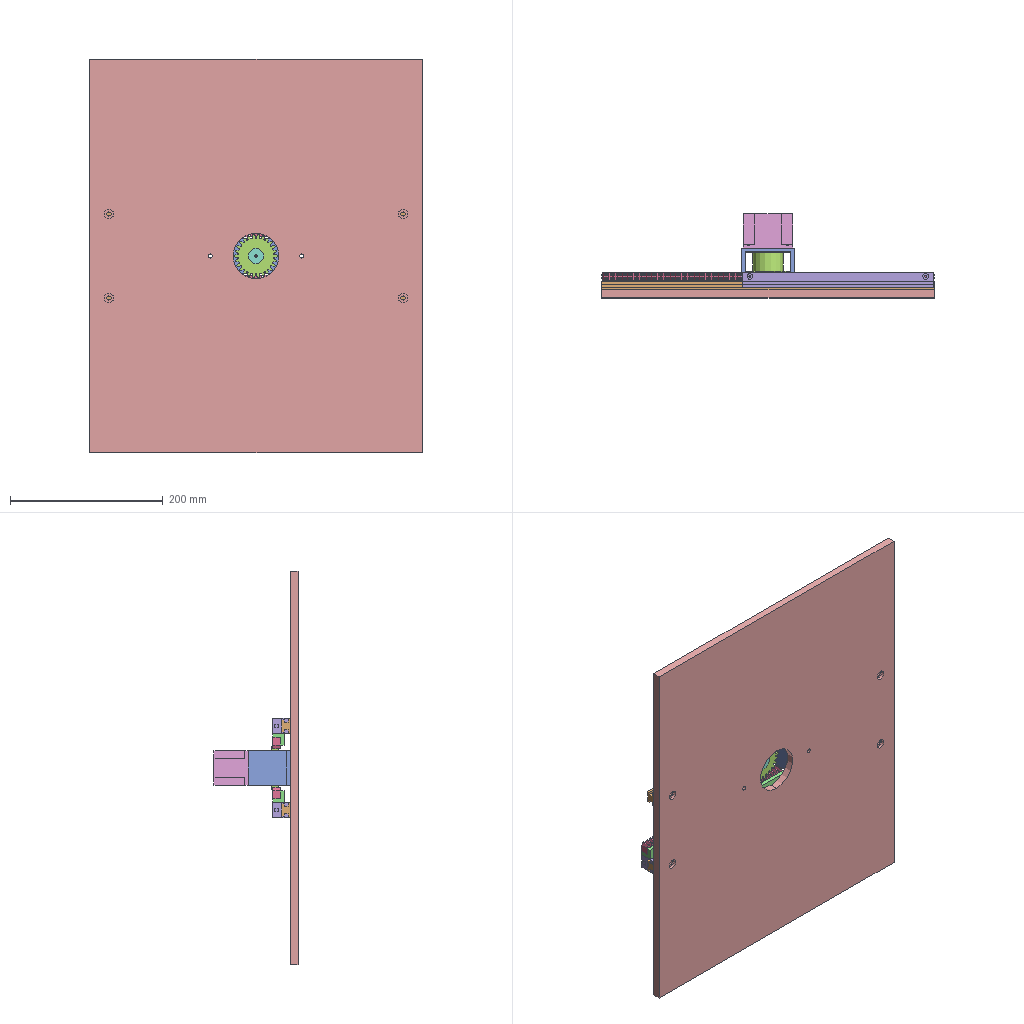Assembly | SolidWorks | 9 different items | 13 placed | box 435 x 110 x 515 mm
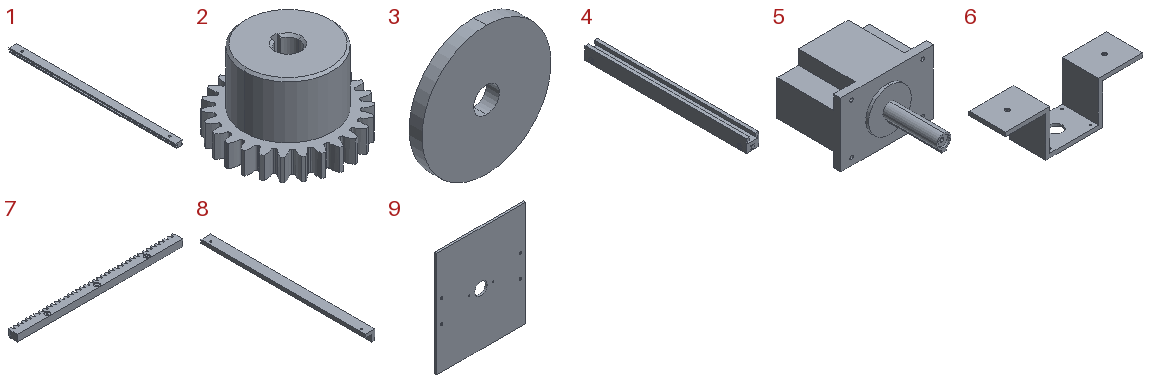Parts list (item | quantity | size | volume | features):
1 | x2 | 20 x 435 x 11 mm | 68492 mm3 | features Extrusion 1, ICE 1
2 | x1 | 56 x 55.747 x 35 mm | 49300 mm3 | features ICE 4, Chamfer 1, CirPattern 1, Extrusion 1, RefAxis 1
3 | x1 | 20 x 2 x 20 mm | 603.186 mm3 | features Extrusion 1
4 | x2 | 20 x 252.4 x 20 mm | 75264 mm3 | features ICE 3, Extrusion 1, HoleWzd 1
5 | x1 | 65 x 85 x 45 mm | 111801 mm3 | features ICE 4, HoleWzd 2, Extrusion 1
6 | x1 | 170 x 45 x 55 mm | 57748 mm3 | features ICE 2, Cut 1, Extrusion 1, HoleWzd 1
7 | x2 | 250.006 x 14.5 x 10 mm | 30674 mm3 | features Boss 1, Extrusion 1, HoleWzd 1, LPattern 1
8 | x2 | 15 x 250 x 15 mm | 31137 mm3 | features Cut 2, Extrusion 1
9 | x1 | 435 x 10 x 515 mm | 2209236 mm3 | features ICE 2, Extrusion 1, HoleWzd 1
Mates (type | each side: item.copy, entity, surface, feature):
Coincident | 9.1 face plane Boss-Extrude1 | 6.1 face plane Boss-Extrude3
Concentric | 9.1 edge | 6.1 edge | 2 times
Coincident | 6.1 face plane Boss-Extrude3 | 2.1 face plane Boss-Extrude3
Concentric | 2.1 face cylinder Cut-Extrude5 | 5.1 face cylinder Boss-Extrude2
Coincident | 2.1 face plane Cut-Extrude6 | 5.1 face plane Boss-Extrude3
Coincident | 6.1 face plane Boss-Extrude3 | 5.1 face plane Boss-Extrude1
Concentric | 6.1 edge | 5.1 edge
Concentric | 5.1 select_type:24 | 3.1 edge
Coincident | 2.1 face plane Boss-Extrude1 | 3.1 face plane Boss-Extrude1
Coincident | 9.1 face plane Boss-Extrude1 | 1.1 face plane Boss-Extrude1 | 2 times
Coincident | 9.1 face plane Boss-Extrude1 | 1.2 face plane Boss-Extrude1 | 2 times
Coincident | 1.1 face plane Boss-Extrude1 | 4.1 face plane Boss-Extrude1 | 2 times
Coincident | 1.2 face plane Boss-Extrude1 | 4.2 face plane Boss-Extrude1 | 2 times
Coincident | 4.2 face plane Boss-Extrude1 | 8.1 face plane Boss-Extrude1 | 3 times
Coincident | 8.1 face plane Boss-Extrude1 | 7.1 face plane Extrude1 | 3 times
Coincident | 7.2 face plane Extrude1 | 8.2 face plane Boss-Extrude1
Coincident | 8.2 face plane Boss-Extrude1 | 7.2 face plane Extrude1
Coincident | 8.2 edge | 7.2 face cylinder CBORE for M2 Hex Cap Screw1 | 2 times
Concentric | 4.1 edge | 8.2 face cylinder Cut-Extrude2
Coincident | 4.1 edge | 8.2 face cylinder Cut-Extrude2
Coincident | 4.1 face plane Boss-Extrude1 | 8.2 face plane Boss-Extrude1
Concentric | 9.1 edge | 1.2 edge
Concentric | 9.1 edge | 1.1 edge
Parallel | 6.1 face plane Boss-Extrude3 | 5.1 face plane Boss-Extrude1
RackPinionDim | 7.2 select_type:24 | 2.1 select_type:24
RackPinionDim | 7.1 select_type:24 | 2.1 select_type:24